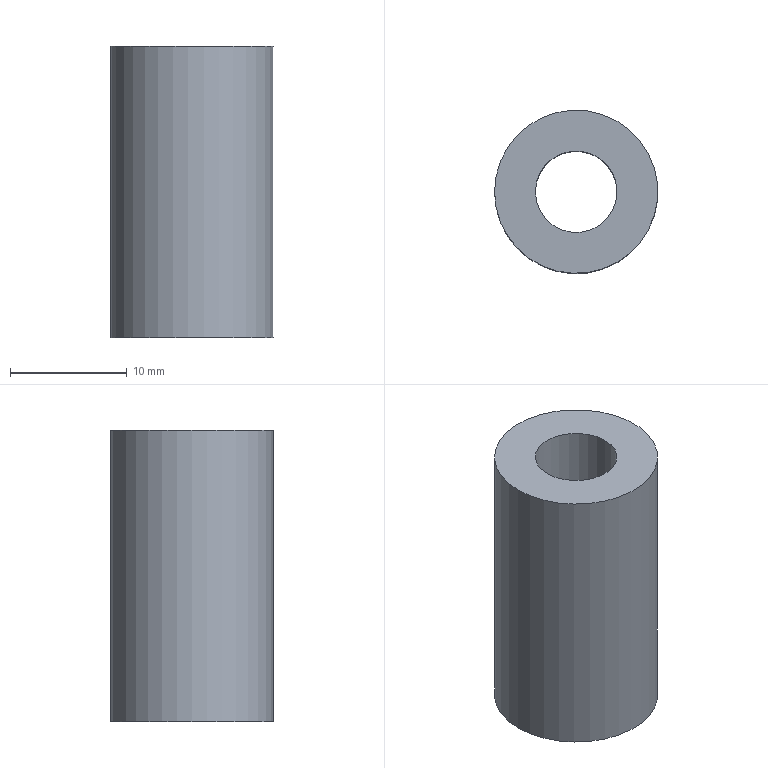Part | NX | features solid 2 | 1 solid | 4 faces | box 14 x 14 x 25 mm | volume 2886 mm3 | cylinder 2 | plane 2 | commonest cylinder face diameters 7 x1 14 x1
STEP:
#1=CARTESIAN_POINT('',(428.006,28.27,7.));
#2=VERTEX_POINT('',#1);
#3=CARTESIAN_POINT('',(435.006,28.27,7.));
#4=DIRECTION('',(0.,0.,-1.));
#5=DIRECTION('',(-1.,0.,0.));
#6=AXIS2_PLACEMENT_3D('',#3,#4,#5);
#7=CIRCLE('',#6,7.);
#8=EDGE_CURVE('',#2,#2,#7,.T.);
#9=ORIENTED_EDGE('',*,*,#8,.T.);
#10=EDGE_LOOP('',(#9));
#11=FACE_BOUND('',#10,.T.);
#12=CARTESIAN_POINT('',(428.006,28.27,-18.));
#13=VERTEX_POINT('',#12);
#14=CARTESIAN_POINT('',(435.006,28.27,-18.));
#15=DIRECTION('',(0.,0.,-1.));
#16=DIRECTION('',(-1.,0.,0.));
#17=AXIS2_PLACEMENT_3D('',#14,#15,#16);
#18=CIRCLE('',#17,7.);
#19=EDGE_CURVE('',#13,#13,#18,.T.);
#20=ORIENTED_EDGE('',*,*,#19,.F.);
#21=EDGE_LOOP('',(#20));
#22=FACE_BOUND('',#21,.T.);
#23=CARTESIAN_POINT('',(435.006,28.27,7.));
#24=DIRECTION('',(0.,0.,-1.));
#25=DIRECTION('',(1.,0.,0.));
#26=AXIS2_PLACEMENT_3D('',#23,#24,#25);
#27=CYLINDRICAL_SURFACE('',#26,7.);
#28=ADVANCED_FACE('',(#11,#22),#27,.T.);
#29=CARTESIAN_POINT('',(431.506,28.27,7.));
#30=VERTEX_POINT('',#29);
#31=CARTESIAN_POINT('',(435.006,28.27,7.));
#32=DIRECTION('',(0.,0.,-1.));
#33=DIRECTION('',(-1.,0.,0.));
#34=AXIS2_PLACEMENT_3D('',#31,#32,#33);
#35=CIRCLE('',#34,3.5);
#36=EDGE_CURVE('',#30,#30,#35,.T.);
#37=ORIENTED_EDGE('',*,*,#36,.T.);
#38=EDGE_LOOP('',(#37));
#39=FACE_BOUND('',#38,.T.);
#40=ORIENTED_EDGE('',*,*,#8,.F.);
#41=EDGE_LOOP('',(#40));
#42=FACE_BOUND('',#41,.T.);
#43=CARTESIAN_POINT('',(435.006,28.27,7.));
#44=DIRECTION('',(0.,0.,1.));
#45=DIRECTION('',(-1.,0.,0.));
#46=AXIS2_PLACEMENT_3D('',#43,#44,#45);
#47=PLANE('',#46);
#48=ADVANCED_FACE('',(#39,#42),#47,.T.);
#49=CARTESIAN_POINT('',(431.506,28.27,-18.));
#50=VERTEX_POINT('',#49);
#51=CARTESIAN_POINT('',(435.006,28.27,-18.));
#52=DIRECTION('',(0.,0.,-1.));
#53=DIRECTION('',(-1.,0.,0.));
#54=AXIS2_PLACEMENT_3D('',#51,#52,#53);
#55=CIRCLE('',#54,3.5);
#56=EDGE_CURVE('',#50,#50,#55,.T.);
#57=ORIENTED_EDGE('',*,*,#56,.F.);
#58=EDGE_LOOP('',(#57));
#59=FACE_BOUND('',#58,.T.);
#60=ORIENTED_EDGE('',*,*,#19,.T.);
#61=EDGE_LOOP('',(#60));
#62=FACE_BOUND('',#61,.T.);
#63=CARTESIAN_POINT('',(435.006,28.27,-18.));
#64=DIRECTION('',(0.,0.,1.));
#65=DIRECTION('',(-1.,0.,0.));
#66=AXIS2_PLACEMENT_3D('',#63,#64,#65);
#67=PLANE('',#66);
#68=ADVANCED_FACE('',(#59,#62),#67,.F.);
#69=ORIENTED_EDGE('',*,*,#36,.F.);
#70=EDGE_LOOP('',(#69));
#71=FACE_BOUND('',#70,.T.);
#72=ORIENTED_EDGE('',*,*,#56,.T.);
#73=EDGE_LOOP('',(#72));
#74=FACE_BOUND('',#73,.T.);
#75=CARTESIAN_POINT('',(435.006,28.27,-18.));
#76=DIRECTION('',(0.,0.,1.));
#77=DIRECTION('',(-1.,0.,0.));
#78=AXIS2_PLACEMENT_3D('',#75,#76,#77);
#79=CYLINDRICAL_SURFACE('',#78,3.5);
#80=ADVANCED_FACE('',(#71,#74),#79,.F.);
#81=CLOSED_SHELL('',(#28,#48,#68,#80));
#82=MANIFOLD_SOLID_BREP('',#81);
#83=(LENGTH_UNIT()NAMED_UNIT(*)SI_UNIT(.MILLI.,.METRE.));
#84=UNCERTAINTY_MEASURE_WITH_UNIT(LENGTH_MEASURE(0.00001),#83,'','');
#85=(NAMED_UNIT(*)PLANE_ANGLE_UNIT()SI_UNIT($,.RADIAN.));
#86=(NAMED_UNIT(*)SI_UNIT($,.STERADIAN.)SOLID_ANGLE_UNIT());
#87=(GEOMETRIC_REPRESENTATION_CONTEXT(3)GLOBAL_UNCERTAINTY_ASSIGNED_CONTEXT((#84))GLOBAL_UNIT_ASSIGNED_CONTEXT((#83,#85,#86))REPRESENTATION_CONTEXT('',''));
#88=ADVANCED_BREP_SHAPE_REPRESENTATION('',(#82),#87);